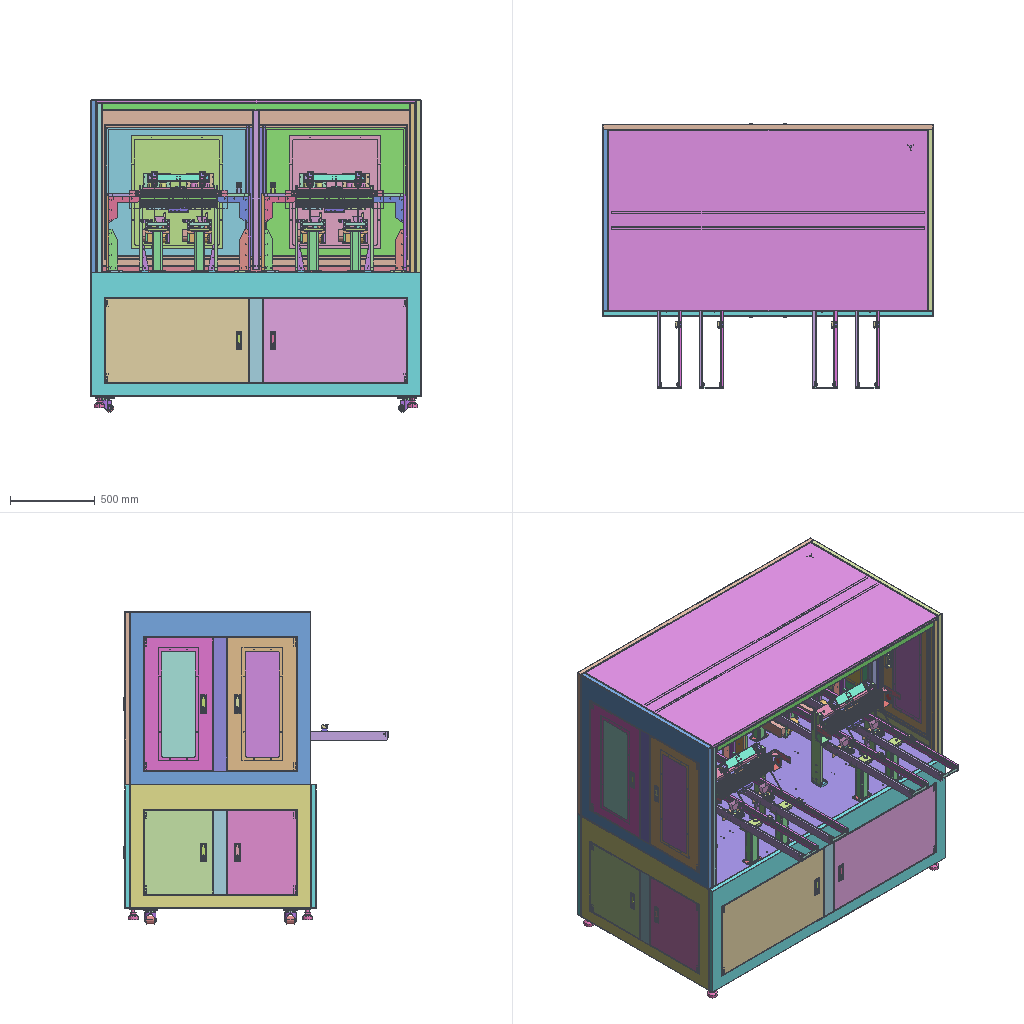Assembly | SolidWorks | 555 different items | 1287 placed | box 1959 x 1559 x 1844 mm
Parts list (item | name | quantity | parent item | size | volume | features), first 326 of 555 items:
1 | 170 Bar Light (subassembly) | x1 | - | - | - | -
2 | (subassembly) | x1 | - | - | - | -
3 | (subassembly) | x1 | - | - | - | -
4 | (subassembly) | x1 | - | - | - | -
5 | (subassembly) | x1 | - | - | - | -
6 | (subassembly) | x1 | - | - | - | -
7 | (subassembly) | x1 | - | - | - | -
8 | (subassembly) | x1 | - | - | - | -
9 | (subassembly) | x1 | - | - | - | -
10 | (subassembly) | x1 | - | - | - | -
11 | (subassembly) | x2 | in 100 | 36 x 22.6 x 446 mm | 126686 mm3 | -
12 | (subassembly) | x1 | - | 36 x 22.6 x 446 mm | 126686 mm3 | -
13 | (subassembly) | x2 | in 102 | 36 x 22.6 x 446 mm | 126686 mm3 | -
14 | (subassembly) | x1 | - | 36 x 22.6 x 446 mm | 126686 mm3 | -
15 | (subassembly) | x2 | in 11 | 36 x 22.6 x 446 mm | 126686 mm3 | -
16 | (subassembly) | x1 | - | 36 x 22.6 x 446 mm | 126686 mm3 | -
17 | (subassembly) | x2 | in 13 | 36 x 22.6 x 446 mm | 126686 mm3 | -
18 | (subassembly) | x1 | - | 36 x 22.6 x 446 mm | 126686 mm3 | -
19 | (subassembly) | x5 | in 41, 42, 106, 107 | 18 x 8 x 56 mm | 2050 mm3 | -
20 | (subassembly) | x5 | in 41, 42, 106, 107 | 18 x 8 x 56 mm | 2050 mm3 | -
21 | (subassembly) | x1 | - | 167.4 x 156.1 x 106 mm | 703605 mm3 | -
22 | (subassembly) | x4 | in 36 | - | 52174 mm3 | -
23 | (subassembly) | x1 | - | - | 52174 mm3 | -
24 | (subassembly) | x1 | - | 54.801 x 54.801 x 36 mm | 20137 mm3 | -
25 | (subassembly) | x1 | - | 26.4 x 61 x 95 mm | 91411 mm3 | -
26 | (subassembly) | x1 | - | 62 x 40 x 105 mm | 103479 mm3 | -
27 | (subassembly) | x4 | in 44 | 110 x 100.5 x 78.14 mm | 89945 mm3 | -
28 | (subassembly) | x4 | in 44 | 40 x 20 x 42 mm | 13632 mm3 | -
29 | (subassembly) | x4 | in 62 | 60 x 143 x 60 mm | 120514 mm3 | -
30 | (subassembly) | x1 | - | 55.81 x 44 x 17.63 mm | 3255 mm3 | -
31 | (subassembly) | x2 | in 34 | - | 422157 mm3 | -
32 | (subassembly) | x4 | in 27 | 29.349 x 29.349 x 44 mm | 30226 mm3 | -
33 | (subassembly) | x4 | in 31 | 39.5 x 98.192 x 39.5 mm | 79084 mm3 | -
34 | (subassembly) | x2 | - | - | 2173391 mm3 | -
35 | (subassembly) | x1 | in 63 | 1886 x 1068 x 18.5 mm | 3707477 mm3 | -
36 | (subassembly) | x4 | in 60 | - | 91199 mm3 | -
37 | (subassembly) | x1 | - | - | 91199 mm3 | -
38 | (subassembly) | x2 | in 58 | 460 x 515 x 80 mm | 1818663 mm3 | -
39 | (subassembly) | x1 | - | 460 x 515 x 80 mm | 1818663 mm3 | features InContextFeatHolder 8
40 | (subassembly) | x2 | in 34 | 380 x 465 x 80 mm | 1262568 mm3 | -
41 | (subassembly) | x1 | in 63 | 851 x 799 x 42.5 mm | 2246546 mm3 | -
42 | (subassembly) | x1 | in 63 | 411 x 799 x 42.5 mm | 1154283 mm3 | -
43 | (subassembly) | x1 | - | 37 x 32 x 81 mm | 32994 mm3 | -
44 | (subassembly) | x4 | - | - | 4376702 mm3 | features Belt 2, AEMSimFeature 1, CompositeCurve 1
45 | (subassembly) | x2 | in 34 | 180 x 151.4 x 77.5 mm | 341470 mm3 | -
46 | (subassembly) | x2 | in 34 | 80 x 78 x 120 mm | 142531 mm3 | -
47 | (subassembly) | x1 | in 62 | 1870 x 1060 x 100 mm | 196301866 mm3 | -
48 | (subassembly) | x20 | in 44 | 26 x 27 x 27 mm | 5259 mm3 | -
49 | (subassembly) | x16 | in 44 | 15 x 27 x 27 mm | 4689 mm3 | -
50 | (subassembly) | x1 | - | 184.199 x 51.718 x 52 mm | 174648 mm3 | features InContextFeatHolder 2
51 | (subassembly) | x2 | in 58 | - | 517771 mm3 | -
52 | (subassembly) | x1 | - | - | 517771 mm3 | -
53 | (subassembly) | x1 | - | - | - | features InContextFeatHolder 9
54 | (subassembly) | x4 | in 62 | 82 x 84 x 107 mm | 193341 mm3 | -
55 | (subassembly) | x1 | - | - | - | features InContextFeatHolder 9
56 | (subassembly) | x1 | - | - | - | features InContextFeatHolder 16
57 | (subassembly) | x1 | - | - | - | features InContextFeatHolder 16
58 | (subassembly) | x2 | - | - | - | features CompositeCurve 1
59 | (subassembly) | x1 | - | - | - | features InContextFeatHolder 4, CompositeCurve 1
60 | (subassembly) | x2 | in 58 | - | 394201 mm3 | features LocalLPattern 1, ReferencePattern 1
61 | (subassembly) | x1 | - | - | 394201 mm3 | features InContextFeatHolder 2, LocalLPattern 1, ReferencePattern 1
62 | (subassembly) | x1 | - | - | 240689348 mm3 | features ReferencePattern 27, LocalLPattern 6, MirrorCompFeat 6
63 | (subassembly) | x1 | in 62 | - | 22995452 mm3 | features ReferencePattern 6, MirrorCompFeat 4
64 | (subassembly) | x2 | in 62 | 1950 x 730 x 42.5 mm | 3302134 mm3 | features MirrorCompFeat 1, ReferencePattern 1
65 | (subassembly) | x1 | - | 195 x 25 x 42 mm | 20018 mm3 | -
66 | (subassembly) | x1 | - | 107.648 x 234.199 x 214.156 mm | 253292 mm3 | features CompositeCurve 1
67 | (subassembly) | x1 | - | 150 x 155 x 181.5 mm | 514877 mm3 | features AEMSimFeature 1
68 | (subassembly) | x2 | in 104 | 306 x 42 x 30 mm | 21853 mm3 | -
69 | (subassembly) | x1 | - | 306 x 42 x 30 mm | 21853 mm3 | -
70 | (subassembly) | x2 | in 100 | 450 x 42 x 35 mm | 35252 mm3 | -
71 | (subassembly) | x1 | - | 450 x 42 x 35 mm | 35252 mm3 | features InContextFeatHolder 2
72 | (subassembly) | x2 | in 97 | 18 x 8 x 56 mm | 2050 mm3 | -
73 | (subassembly) | x1 | in 99 | 18 x 8 x 56 mm | 2050 mm3 | -
74 | (subassembly) | x2 | in 96 | 18 x 8 x 56 mm | 2050 mm3 | -
75 | (subassembly) | x2 | in 92 | 18 x 8 x 56 mm | 2050 mm3 | -
76 | (subassembly) | x2 | in 104 | 36 x 22.6 x 302 mm | 86992 mm3 | -
77 | (subassembly) | x1 | in 91 | 18 x 8 x 56 mm | 2050 mm3 | -
78 | (subassembly) | x1 | in 93 | 18 x 8 x 56 mm | 2050 mm3 | -
79 | (subassembly) | x2 | in 97 | 18 x 8 x 56 mm | 2050 mm3 | -
80 | (subassembly) | x1 | in 99 | 18 x 8 x 56 mm | 2050 mm3 | -
81 | (subassembly) | x2 | in 96 | 18 x 8 x 56 mm | 2050 mm3 | -
82 | (subassembly) | x2 | in 92 | 18 x 8 x 56 mm | 2050 mm3 | -
83 | (subassembly) | x1 | in 91 | 18 x 8 x 56 mm | 2050 mm3 | -
84 | (subassembly) | x1 | in 93 | 18 x 8 x 56 mm | 2050 mm3 | -
85 | (subassembly) | x2 | in 89 | - | 428016 mm3 | -
86 | (subassembly) | x2 | in 85 | 39.5 x 98.192 x 39.5 mm | 82462 mm3 | -
87 | (subassembly) | x1 | - | 36 x 22.6 x 302 mm | 86992 mm3 | -
88 | (subassembly) | x2 | in 85 | 39.5 x 98.192 x 39.5 mm | 82462 mm3 | -
89 | (subassembly) | x2 | - | - | 2167435 mm3 | -
90 | (subassembly) | x2 | in 89 | 380 x 465 x 80 mm | 1262568 mm3 | -
91 | (subassembly) | x1 | in 63 | 851 x 799 x 42.5 mm | 2246546 mm3 | -
92 | (subassembly) | x2 | in 63 | 411 x 799 x 42.5 mm | 1154283 mm3 | -
93 | (subassembly) | x1 | in 63 | 411 x 799 x 42.5 mm | 1154283 mm3 | -
94 | (subassembly) | x2 | in 89 | 180 x 151.4 x 77.5 mm | 341470 mm3 | -
95 | (subassembly) | x2 | in 89 | 80 x 78 x 120 mm | 142531 mm3 | -
96 | (subassembly) | x2 | in 64 | 851 x 509 x 42.5 mm | 870098 mm3 | -
97 | (subassembly) | x2 | in 62 | 411 x 509 x 42.5 mm | 486734 mm3 | -
98 | (subassembly) | x1 | - | 36 x 22.6 x 302 mm | 86992 mm3 | -
99 | (subassembly) | x1 | in 62 | 411 x 509 x 42.5 mm | 486734 mm3 | -
100 | (subassembly) | x2 | in 51 | - | 230759 mm3 | -
101 | (subassembly) | x1 | - | - | 230759 mm3 | -
102 | (subassembly) | x2 | in 51 | - | 224548 mm3 | -
103 | (subassembly) | x1 | - | - | 224548 mm3 | -
104 | (subassembly) | x2 | in 51 | 306 x 50.679 x 130.275 mm | 162971 mm3 | -
105 | (subassembly) | x1 | - | 306 x 50.679 x 130.275 mm | 162971 mm3 | -
106 | (subassembly) | x2 | in 64 | 851 x 509 x 42.5 mm | 870098 mm3 | -
107 | (subassembly) | x1 | in 62 | 411 x 509 x 42.5 mm | 486734 mm3 | -
108 | - | x1 | - | 1386 x 30 x 15 mm | 332572 mm3 | features HoleWzd 2, 3DProfileFeature 1, ICE 1, WeldMemberFeat 1, WeldmentFeature 1
109 | - | x4 | in 28 | 12 x 11 x 15 mm | 1507 mm3 | features ICE 5, Chamfer 2, Extrusion 1
110 | - | x4 | in 28 | 40 x 20 x 16 mm | 7506 mm3 | features HoleWzd 2, Chamfer 1, Extrusion 1, ICE 1
111 | - | x1 | - | 1087 x 374 x 123 mm | 809461 mm3 | features ICE 4, Fillet 2, EdgeFlange 1, FlatPattern 1, SMBaseFlange 1, SheetMetal 1
112 | - | x1 | - | 1087 x 374 x 1.5 mm | 609421 mm3 | features Fillet 1, FlatPattern 1, ICE 1, SMBaseFlange 1, SheetMetal 1
113 | - | x1 | - | 1280 x 374 x 1.5 mm | 717635 mm3 | features Fillet 1, FlatPattern 1, HoleWzd 1, SMBaseFlange 1, SheetMetal 1
114 | - | x1 | - | 10 x 145 x 145 mm | 203124 mm3 | features HoleWzd 2, ICE 2, Chamfer 1, Extrusion 1
115 | - | x1 | - | 100 x 301.5 x 60 mm | 406752 mm3 | features Chamfer 4, ICE 4, HoleWzd 2, 3DProfileFeature 1, WeldMemberFeat 1, WeldmentFeature 1
116 | - | x1 | - | 20 x 410 x 40 mm | 242107 mm3 | features ICE 3, Chamfer 1, Extrusion 1, HoleWzd 1
117 | - | x1 | - | 317 x 30 x 11 mm | 98288 mm3 | features Chamfer 2, HoleWzd 2, Extrusion 1, ICE 1
118 | - | x1 | - | 317 x 15 x 170 mm | 619521 mm3 | features ICE 5, HoleWzd 4, Chamfer 2, Extrusion 1, Fillet 1
119 | - | x1 | - | 805 x 30 x 15 mm | 189619 mm3 | features 3DProfileFeature 1, HoleWzd 1, ICE 1, WeldMemberFeat 1, WeldmentFeature 1
120 | - | x1 | - | 317 x 8 x 29 mm | 69848 mm3 | features HoleWzd 2, ICE 2, Chamfer 1, Extrusion 1
121 | - | x1 | - | 297 x 3 x 90 mm | 79946 mm3 | features Chamfer 3, Extrusion 1, HoleWzd 1
122 | - | x1 | - | 30 x 30 x 10 mm | 7510 mm3 | features Chamfer 2, Extrusion 1, HoleWzd 1, ICE 1
123 | - | x1 | - | 18 x 14 x 15 mm | 1893 mm3 | features ICE 2, Chamfer 1, Extrusion 1, HoleWzd 1
124 | - | x1 | - | 62 x 8 x 20 mm | 9069 mm3 | features Chamfer 1, Extrusion 1, HoleWzd 1
125 | - | x1 | - | 20 x 20 x 415 mm | 128650 mm3 | features HoleWzd 2, Chamfer 1, Extrusion 1
126 | - | x1 | - | 210 x 12 x 280 mm | 525634 mm3 | features ICE 4, Chamfer 3, Extrusion 1, Fillet 1
127 | - | x1 | - | 35 x 15 x 40 mm | 12452 mm3 | features Chamfer 1, Extrusion 1, HoleWzd 1, ICE 1
128 | - | x1 | - | 48 x 133 x 30 mm | 14568 mm3 | features CornerTrim 2, ICE 2, FlatPattern 1, HoleWzd 1, SMBaseFlange 1, SheetMetal 1
129 | - | x1 | - | 50 x 30 x 15 mm | 18955 mm3 | features Chamfer 2, Extrusion 1, HoleWzd 1
130 | - | x1 | - | 1386 x 30 x 15 mm | 334202 mm3 | features 3DProfileFeature 1, HoleWzd 1, ICE 1, WeldMemberFeat 1, WeldmentFeature 1
131 | - | x1 | - | 50 x 30 x 15 mm | 18955 mm3 | features Chamfer 2, Extrusion 1, HoleWzd 1
132 | - | x1 | - | 40 x 30 x 15 mm | 15105 mm3 | features Chamfer 1, Extrusion 1, HoleWzd 1
133 | - | x1 | - | 20 x 16 x 20 mm | 4067 mm3 | features HoleWzd 2, Chamfer 1, Extrusion 1, ICE 1
134 | - | x1 | - | 20 x 16 x 20 mm | 4064 mm3 | features HoleWzd 2, Chamfer 1, Extrusion 1, ICE 1
135 | - | x1 | - | 28 x 12 x 18 mm | 4573 mm3 | features Chamfer 1, Extrusion 1, HoleWzd 1
136 | - | x1 | - | 330 x 10 x 30 mm | 97693 mm3 | features Chamfer 1, Extrusion 1, HoleWzd 1
137 | - | x1 | - | 30 x 40 x 40 mm | 21456 mm3 | features Chamfer 3, ICE 2, Extrusion 1, HoleWzd 1
138 | - | x1 | - | 40 x 320 x 40 mm | 193550 mm3 | features WeldMemberFeat 1, WeldmentFeature 1
139 | - | x1 | - | 39 x 35 x 33 mm | 21329 mm3 | features HoleWzd 2, Chamfer 1, Extrusion 1, ICE 1
140 | - | x1 | - | 16.5 x 26.5 x 35 mm | 1824 mm3 | features ICE 2, Chamfer 1, FlatPattern 1, SMBaseFlange 1, SheetMetal 1
141 | - | x1 | - | 805 x 30 x 15 mm | 190827 mm3 | features 3DProfileFeature 1, HoleWzd 1, ICE 1, WeldMemberFeat 1, WeldmentFeature 1
142 | - | x1 | - | 50 x 5 x 30 mm | 6223 mm3 | features ICE 3, Chamfer 2, HoleWzd 2, CornerTrim 1, FlatPattern 1, SMBaseFlange 1, SheetMetal 1
143 | - | x1 | - | 1283 x 1093 x 1.5 mm | 2101440 mm3 | features HoleWzd 2, Cut 1, Extrusion 1, Fillet 1
144 | - | x1 | - | 30 x 40 x 200 mm | 67180 mm3 | features Chamfer 2, HoleWzd 2, Extrusion 1, ICE 1
145 | - | x1 | - | 140 x 539 x 60 mm | 688528 mm3 | features Chamfer 3, ICE 3, HoleWzd 2, 3DProfileFeature 1, WeldMemberFeat 1, WeldmentFeature 1
146 | - | x1 | - | 1000 x 60 x 20 mm | 1185060 mm3 | features Chamfer 2, HoleWzd 2, Extrusion 1, LPattern 1
147 | - | x1 | - | 80 x 379 x 120 mm | 535710 mm3 | features HoleWzd 4, Chamfer 2, ICE 2, WeldMemberFeat 1, WeldmentFeature 1
148 | - | x1 | - | 633 x 12 x 86.5 mm | 646529 mm3 | features HoleWzd 6, Cut 5, ICE 3, Chamfer 2, LPattern 2, Extrusion 1
149 | - | x1 | - | 680 x 45 x 10 mm | 288393 mm3 | features HoleWzd 10, Chamfer 2, Cut 1, Extrusion 1, LPattern 1
150 | - | x1 | - | 64 x 102 x 19 mm | 119355 mm3 | features HoleWzd 4, Chamfer 2, Cut 1, Extrusion 1, ICE 1
151 | - | x1 | - | 130 x 84 x 12 mm | 83062 mm3 | features ICE 8, Chamfer 3, HoleWzd 3, Cut 2, Extrusion 1
152 | - | x1 | - | 10 x 14 x 10 mm | 408.891 mm3 | features Chamfer 3, ICE 3, Extrusion 1
153 | - | x1 | - | 72 x 98 x 40 mm | 71413 mm3 | features HoleWzd 3, Chamfer 2, Cut 1, Extrusion 1, Fillet 1
154 | - | x1 | - | 50 x 30 x 10 mm | 12561 mm3 | features HoleWzd 2, Chamfer 1, Extrusion 1
155 | - | x1 | - | 42 x 59 x 21 mm | 26880 mm3 | features ICE 4, Chamfer 2, HoleWzd 2, Extrusion 1
156 | - | x1 | - | 20 x 19.9 x 54 mm | 6398 mm3 | features ICE 8, HoleWzd 3, Extrusion 1
157 | - | x1 | - | 30 x 24.5 x 29.5 mm | 1040 mm3 | features Fillet 3, ICE 3, EdgeFlange 2, Cut 1, FlatPattern 1, SMBaseFlange 1, SheetMetal 1
158 | - | x1 | - | 110 x 85 x 4 mm | 36598 mm3 | features HoleWzd 2, Chamfer 1, Extrusion 1
159 | - | x1 | - | 110 x 85 x 2 mm | 15306 mm3 | features ICE 15, HoleWzd 5, MoveFace 2, Chamfer 1, Cut 1, Extrusion 1, Fillet 1, MirrorPattern 1
160 | - | x1 | - | 30 x 85 x 29 mm | 7084 mm3 | features EdgeFlange 3, HoleWzd 2, FlatPattern 1, SMBaseFlange 1, SheetMetal 1
161 | - | x1 | - | 77 x 33 x 22 mm | 5955 mm3 | features EdgeFlange 2, HoleWzd 2, Chamfer 1, FlatPattern 1, ICE 1, SMBaseFlange 1, SheetMetal 1
162 | - | x1 | - | 64 x 14 x 87 mm | 75198 mm3 | features HoleWzd 2, Chamfer 1, Extrusion 1
163 | - | x2 | in 104 | 120 x 128.5 x 45 mm | 54126 mm3 | features HoleWzd 3, EdgeFlange 2, Fillet 1, FlatPattern 1, ICE 1, SMBaseFlange 1, SheetMetal 1
164 | - | x1 | - | 8 x 70 x 8 mm | 3389 mm3 | features Chamfer 1, Extrusion 1, HoleWzd 1
165 | - | x1 | - | 10 x 90 x 58 mm | 50238 mm3 | features HoleWzd 2, Chamfer 1, Extrusion 1
166 | - | x1 | - | 110 x 85 x 4 mm | 36664 mm3 | features HoleWzd 2, Chamfer 1, Extrusion 1
167 | - | x1 | - | 24 x 8 x 170 mm | 30923 mm3 | features Chamfer 2, HoleWzd 2, Extrusion 1
168 | - | x1 | - | 110 x 85 x 6 mm | 53736 mm3 | features HoleWzd 2, Chamfer 1, Extrusion 1
169 | - | x1 | - | 64 x 130 x 10 mm | 78799 mm3 | features HoleWzd 2, Chamfer 1, Extrusion 1
170 | - | x1 | - | 74 x 216 x 12 mm | 104830 mm3 | features Chamfer 2, HoleWzd 2, Cut 1, Extrusion 1
171 | - | x1 | - | 12 x 68 x 33 mm | 24708 mm3 | features HoleWzd 3, Chamfer 1, Extrusion 1
172 | - | x1 | - | 25 x 36 x 10 mm | 6742 mm3 | features HoleWzd 2, Chamfer 1, Extrusion 1
173 | - | x1 | - | 60 x 72 x 12 mm | 45188 mm3 | features HoleWzd 2, Chamfer 1, Extrusion 1
174 | - | x1 | - | 120 x 128.5 x 45 mm | 54126 mm3 | features HoleWzd 3, EdgeFlange 2, Fillet 1, FlatPattern 1, ICE 1, SMBaseFlange 1, SheetMetal 1
175 | - | x1 | - | 870 x 90 x 10 mm | 777394 mm3 | features HoleWzd 4, Chamfer 1, Extrusion 1, ICE 1, LPattern 1
176 | - | x1 | - | 20 x 20 x 4 mm | 1002 mm3 | features Extrusion 1
177 | - | x1 | - | 12 x 28 x 68 mm | 21134 mm3 | features Chamfer 2, HoleWzd 2, Extrusion 1
178 | - | x1 | - | 110 x 85 x 2 mm | 15729 mm3 | features Cut 2, Extrusion 1
179 | - | x4 | in 44 | 20 x 50 x 1500 mm | 1167448 mm3 | features HoleWzd 7, Cut 3, Chamfer 2, ICE 2, Extrusion 1, Fillet 1
180 | - | x8 | in 44 | 100 x 250.5 x 60 mm | 355325 mm3 | features Chamfer 2, HoleWzd 2, ICE 2, 3DProfileFeature 1, WeldMemberFeat 1, WeldmentFeature 1
181 | - | x8 | in 44 | 60 x 13 x 144 mm | 107062 mm3 | features HoleWzd 2, Chamfer 1, Extrusion 1
182 | - | x4 | in 44 | 20 x 50 x 1500 mm | 1170334 mm3 | features HoleWzd 7, ICE 4, Chamfer 2, Extrusion 1, Fillet 1
183 | - | x4 | in 44 | 144 x 35 x 5 mm | 17146 mm3 | features Chamfer 1, Extrusion 1, Fillet 1, HoleWzd 1, ICE 1
184 | - | x4 | in 44 | 30 x 33 x 144 mm | 12527 mm3 | features Fillet 3, ICE 2, Cut 1, Extrusion 1, Shell 1
185 | - | x5 | in 41, 42, 106, 107 | 35 x 42.5 x 110 mm | 68844 mm3 | features BaseBody 1
186 | - | x2 | in 15 | 36 x 15 x 6 mm | 2540 mm3 | features BaseBody 1
187 | - | x1 | - | 36 x 15 x 6 mm | 2540 mm3 | features BaseBody 1
188 | - | x2 | in 17 | 36 x 15 x 6 mm | 2540 mm3 | features BaseBody 1
189 | - | x1 | - | 36 x 15 x 6 mm | 2540 mm3 | features BaseBody 1
190 | - | x2 | in 76 | 36 x 15 x 6 mm | 2540 mm3 | features BaseBody 1
191 | - | x1 | - | 36 x 15 x 6 mm | 2540 mm3 | features BaseBody 1
192 | - | x1 | - | 36 x 15 x 6 mm | 2540 mm3 | features BaseBody 1
193 | - | x2 | in 15 | 36 x 15 x 6 mm | 2606 mm3 | features BaseBody 1
194 | - | x1 | - | 36 x 15 x 6 mm | 2606 mm3 | features BaseBody 1
195 | - | x2 | in 17 | 36 x 15 x 6 mm | 2606 mm3 | features BaseBody 1
196 | - | x1 | - | 40 x 40 x 35 mm | 11668 mm3 | features ICE 3, Extrusion 1
197 | - | x1 | - | 36 x 15 x 6 mm | 2606 mm3 | features BaseBody 1
198 | - | x2 | in 76 | 36 x 15 x 6 mm | 2606 mm3 | features BaseBody 1
199 | - | x1 | - | 36 x 15 x 6 mm | 2606 mm3 | features BaseBody 1
200 | - | x1 | - | 36 x 15 x 6 mm | 2606 mm3 | features BaseBody 1
201 | - | x2 | in 45 | 174 x 1 x 62.5 mm | 10875 mm3 | features BaseBody 1
202 | - | x2 | in 45 | 5 x 105.4 x 62 mm | 29217 mm3 | features BaseBody 1
203 | - | x2 | in 45 | 177 x 36.8 x 1 mm | 6475 mm3 | features BaseBody 1
204 | - | x2 | in 45 | 5 x 105.4 x 62 mm | 29184 mm3 | features BaseBody 1
205 | - | x2 | in 45 | 174 x 6 x 62 mm | 63958 mm3 | features BaseBody 1
206 | - | x2 | in 45 | 174 x 6 x 62 mm | 62898 mm3 | features BaseBody 1
207 | - | x4 | in 100 | 260 x 40 x 130 mm | 34410 mm3 | features HoleWzd 3, EdgeFlange 1, Fillet 1, FlatPattern 1, ICE 1, SMBaseFlange 1, SheetMetal 1
208 | - | x2 | in 45 | 180 x 105.4 x 6 mm | 51969 mm3 | features BaseBody 1
209 | - | x2 | in 45 | 174 x 3 x 62.5 mm | 32625 mm3 | features BaseBody 1
210 | - | x2 | in 45 | 172 x 61 x 61 mm | 14666 mm3 | features BaseBody 1
211 | - | x1 | - | 42 x 17 x 17 mm | 8111 mm3 | features BaseBody 1
212 | - | x4 | in 44 | 16 x 32.358 x 32.358 mm | 6392 mm3 | features ICE 1, Revolution 1
213 | - | x4 | in 44 | 16 x 32.358 x 32.358 mm | 5839 mm3 | features ICE 1, Revolution 1
214 | - | x1 | - | 114 x 47 x 26 mm | 54432 mm3 | features BaseBody 1
215 | - | x1 | - | 158 x 46 x 18 mm | 18569 mm3 | features BaseBody 5
216 | - | x4 | in 33 | 52.8 x 39.5 x 39.5 mm | 57776 mm3 | features Extrusion 1, ICE 1
217 | - | x4 | in 29 | 60 x 143 x 60 mm | 112312 mm3 | features BaseBody 1
218 | - | x1 | - | 39 x 29.5 x 121 mm | 53131 mm3 | features RefAxis 15, HoleWzd 11, ICE 9, 3DProfileFeature 5, LPattern 4, Revolution 3, RevCut 2, Extrusion 1
219 | - | x1 | - | 260 x 40 x 130 mm | 34410 mm3 | features HoleWzd 3, EdgeFlange 1, Fillet 1, FlatPattern 1, ICE 1, SMBaseFlange 1, SheetMetal 1
220 | - | x4 | in 29 | 30 x 16 x 34.641 mm | 8202 mm3 | features BaseBody 1
221 | - | x1 | - | 16.782 x 16 x 17.8 mm | 1225 mm3 | features ICE 4, RefAxis 3, 3DProfileFeature 1, Extrusion 1, Revolution 1
222 | - | x1 | - | 19 x 82 x 28.4 mm | 14487 mm3 | features ICE 12, RefAxis 3, 3DProfileFeature 1, Extrusion 1, Revolution 1
223 | - | x1 | - | 7.2 x 34.2 x 43.1 mm | 5332 mm3 | features RefAxis 9, 3DProfileFeature 3, ICE 2, Extrusion 1
224 | - | x1 | - | 9 x 12 x 9 mm | 395.605 mm3 | features RefAxis 6, 3DProfileFeature 2, Revolution 1
225 | - | x1 | - | 9.996 x 20 x 10 mm | 691.38 mm3 | features BaseBody 1
226 | - | x1 | - | 8 x 32 x 8 mm | 1009 mm3 | features RefAxis 12, 3DProfileFeature 4, Revolution 2, ICE 1, RevCut 1
227 | - | x1 | - | 13.856 x 3 x 12 mm | 252.9 mm3 | features RefAxis 3, 3DProfileFeature 1, ICE 1, Revolution 1
228 | - | x1 | - | 55 x 2 x 14 mm | 1344 mm3 | features RefAxis 3, 3DProfileFeature 1, Extrusion 1
229 | - | x2 | in 76 | 36 x 22.6 x 302 mm | 68970 mm3 | features BaseBody 1
230 | - | x1 | - | 97 x 56.4 x 56.4 mm | 215664 mm3 | features ICE 4, Fillet 2, CirPattern 1, Extrusion 1
231 | - | x1 | - | 36 x 22.6 x 302 mm | 68970 mm3 | features BaseBody 1
232 | - | x1 | - | 36 x 22.6 x 302 mm | 68970 mm3 | features BaseBody 1
233 | - | x2 | in 76 | 31.173 x 7.2 x 23.95 mm | 1073 mm3 | features BaseBody 1
234 | - | x1 | - | 31.173 x 7.2 x 23.95 mm | 1073 mm3 | features BaseBody 1
235 | - | x1 | - | 31.173 x 7.2 x 23.95 mm | 1073 mm3 | features BaseBody 1
236 | - | x2 | in 76 | 31.173 x 7.2 x 23.95 mm | 1073 mm3 | features BaseBody 1
237 | - | x1 | - | 31.173 x 7.2 x 23.95 mm | 1073 mm3 | features BaseBody 1
238 | - | x1 | - | 31.173 x 7.2 x 23.95 mm | 1073 mm3 | features BaseBody 1
239 | - | x2 | in 76 | 31.173 x 7.2 x 23.95 mm | 1073 mm3 | features BaseBody 1
240 | - | x1 | - | 31.173 x 7.2 x 23.95 mm | 1073 mm3 | features BaseBody 1
241 | - | x1 | - | 53 x 45.8 x 53.4 mm | 95835 mm3 | features ICE 7, RefAxis 6, HoleWzd 3, 3DProfileFeature 2, Extrusion 1, LPattern 1, Revolution 1
242 | - | x1 | - | 31.173 x 7.2 x 23.95 mm | 1073 mm3 | features BaseBody 1
243 | - | x2 | in 76 | 31.173 x 7.2 x 23.95 mm | 1073 mm3 | features BaseBody 1
244 | - | x1 | - | 31.173 x 7.2 x 23.95 mm | 1073 mm3 | features BaseBody 1
245 | - | x1 | - | 31.173 x 7.2 x 23.95 mm | 1073 mm3 | features BaseBody 1
246 | - | x2 | in 76 | 31.173 x 7.2 x 23.95 mm | 1073 mm3 | features BaseBody 1
247 | - | x1 | - | 31.173 x 7.2 x 23.95 mm | 1073 mm3 | features BaseBody 1
248 | - | x1 | - | 31.173 x 7.2 x 23.95 mm | 1073 mm3 | features BaseBody 1
249 | - | x2 | in 76 | 31.173 x 7.2 x 23.95 mm | 1073 mm3 | features BaseBody 1
250 | - | x1 | - | 31.173 x 7.2 x 23.95 mm | 1073 mm3 | features BaseBody 1
251 | - | x1 | - | 31.173 x 7.2 x 23.95 mm | 1073 mm3 | features BaseBody 1
252 | - | x1 | - | 19.5 x 11 x 8 mm | 1100 mm3 | features RefAxis 3, Revolution 2, 3DProfileFeature 1, Extrusion 1, HoleWzd 1
253 | - | x2 | in 76 | 31.173 x 7.2 x 23.95 mm | 1073 mm3 | features BaseBody 1
254 | - | x1 | - | 31.173 x 7.2 x 23.95 mm | 1073 mm3 | features BaseBody 1
255 | - | x1 | - | 31.173 x 7.2 x 23.95 mm | 1073 mm3 | features BaseBody 1
256 | - | x2 | in 76 | 31.173 x 7.2 x 23.95 mm | 1073 mm3 | features BaseBody 1
257 | - | x1 | - | 31.173 x 7.2 x 23.95 mm | 1073 mm3 | features BaseBody 1
258 | - | x1 | - | 31.173 x 7.2 x 23.95 mm | 1073 mm3 | features BaseBody 1
259 | - | x2 | in 76 | 31.173 x 7.2 x 23.95 mm | 1073 mm3 | features BaseBody 1
260 | - | x1 | - | 31.173 x 7.2 x 23.95 mm | 1073 mm3 | features BaseBody 1
261 | - | x1 | - | 31.173 x 7.2 x 23.95 mm | 1073 mm3 | features BaseBody 1
262 | - | x2 | in 76 | 31.173 x 7.2 x 23.95 mm | 1073 mm3 | features BaseBody 1
263 | - | x1 | - | 46 x 74.3 x 53 mm | 114802 mm3 | features RefAxis 6, ICE 4, 3DProfileFeature 2, Revolution 1
264 | - | x1 | - | 31.173 x 7.2 x 23.95 mm | 1073 mm3 | features BaseBody 1
265 | - | x1 | - | 31.173 x 7.2 x 23.95 mm | 1073 mm3 | features BaseBody 1
266 | - | x2 | in 76 | 31.173 x 7.2 x 23.95 mm | 1073 mm3 | features BaseBody 1
267 | - | x1 | - | 31.173 x 7.2 x 23.95 mm | 1073 mm3 | features BaseBody 1
268 | - | x1 | - | 31.173 x 7.2 x 23.95 mm | 1073 mm3 | features BaseBody 1
269 | - | x2 | in 76 | 31.173 x 7.2 x 23.95 mm | 1073 mm3 | features BaseBody 1
270 | - | x1 | - | 31.173 x 7.2 x 23.95 mm | 1073 mm3 | features BaseBody 1
271 | - | x1 | - | 31.173 x 7.2 x 23.95 mm | 1073 mm3 | features BaseBody 1
272 | - | x1 | - | 120 x 120 x 38.5 mm | 90385 mm3 | features ICE 3, CirPattern 1, Extrusion 1, Fillet 1, HoleWzd 1, MirrorPattern 1
273 | - | x4 | in 32 | 29.349 x 29.349 x 40.5 mm | 29191 mm3 | features RevCut 4, Extrusion 1, ICE 1
274 | - | x1 | - | 53 x 69.9 x 53.4 mm | 106071 mm3 | features ICE 11, RefAxis 6, HoleWzd 3, 3DProfileFeature 2, Revolution 2, Extrusion 1, LPattern 1
275 | - | x4 | in 36 | 36.008 x 31 x 53.1 mm | 39029 mm3 | features MBimport 1
276 | - | x1 | - | 36.008 x 31 x 53.1 mm | 39029 mm3 | features MBimport 1
277 | - | x4 | in 33 | - | - | features BaseBody 9, RefSurface 2
278 | - | x4 | in 32 | 8 x 8 x 22.5 mm | 1035 mm3 | features ICE 1, RevCut 1, Revolution 1
279 | - | x1 | in 63 | 1950 x 1020 x 48.5 mm | 1634883 mm3 | features EdgeFlange 5, FlatPattern 1, HoleWzd 1, ICE 1, SMBaseFlange 1, SheetMetal 1
280 | - | x1 | in 35 | 1886 x 1068 x 18.5 mm | 3323198 mm3 | features EdgeFlange 2, HoleWzd 2, CirPattern 1, FlatPattern 1, SMBaseFlange 1, SheetMetal 1
281 | - | x1 | in 35 | 110 x 17 x 1845 mm | 384278 mm3 | features FlatPattern 1, SMBaseFlange 1, SheetMetal 1
282 | - | x2 | in 38 | 430 x 80 x 15 mm | 509108 mm3 | features HoleWzd 5, Extrusion 1, MirrorPattern 1
283 | - | x1 | - | 430 x 80 x 15 mm | 509108 mm3 | features HoleWzd 5, Extrusion 1, MirrorPattern 1
284 | - | x4 | in 38 | 80 x 500 x 15 mm | 549882 mm3 | features HoleWzd 4, Extrusion 1, Fillet 1, MirrorPattern 1
285 | - | x1 | - | 46 x 74.3 x 53 mm | 114802 mm3 | features ICE 4, RefAxis 3, 3DProfileFeature 1, Revolution 1
286 | - | x1 | - | 80 x 500 x 15 mm | 549882 mm3 | features HoleWzd 4, Extrusion 1, Fillet 1, MirrorPattern 1
287 | - | x2 | in 40 | 80 x 450 x 15 mm | 533651 mm3 | features HoleWzd 4, Extrusion 1
288 | - | x2 | in 40 | 365 x 80 x 15 mm | 415130 mm3 | features HoleWzd 6, Extrusion 1
289 | - | x1 | - | 238.5 x 96 x 130.5 mm | 1680517 mm3 | features ICE 5, Extrusion 1, Fillet 1
290 | - | x1 | - | 25 x 440 x 25 mm | 214356 mm3 | features Chamfer 1, Extrusion 1, HoleWzd 1
291 | - | x2 | in 15 | 36 x 22.6 x 446 mm | 102225 mm3 | features BaseBody 1
292 | - | x1 | - | 36 x 22.6 x 446 mm | 102225 mm3 | features BaseBody 1
293 | - | x2 | in 17 | 36 x 22.6 x 446 mm | 102225 mm3 | features BaseBody 1
294 | - | x1 | - | 36 x 22.6 x 446 mm | 102225 mm3 | features BaseBody 1
295 | - | x1 | in 62 | 1070 x 730 x 30 mm | 905404 mm3 | features EdgeFlange 4, FlatPattern 1, HoleWzd 1, ICE 1, SMBaseFlange 1, SheetMetal 1
296 | - | x1 | - | 53 x 48.5 x 57 mm | 88299 mm3 | features ICE 8, RefAxis 6, HoleWzd 3, 3DProfileFeature 2, Extrusion 1, RevCut 1, Revolution 1
297 | - | x1 | in 63 | 1070 x 1020 x 48.5 mm | 1078277 mm3 | features EdgeFlange 5, FlatPattern 1, HoleWzd 1, ICE 1, SMBaseFlange 1, SheetMetal 1
298 | - | x4 | in 22 | 4 x 180 x 4 mm | 2262 mm3 | features Extrusion 1
299 | - | x1 | - | 4 x 180 x 4 mm | 2262 mm3 | features Extrusion 1
300 | - | x4 | in 60 | 4 x 300 x 4 mm | 3770 mm3 | features Extrusion 1
301 | - | x1 | - | 4 x 300 x 4 mm | 3770 mm3 | features Extrusion 1
302 | - | x1 | in 41 | 851 x 786 x 26.5 mm | 735444 mm3 | features ICE 4, EdgeFlange 2, MirrorPattern 2, Fillet 1, FlatPattern 1, HoleWzd 1, SMBaseFlange 1, SheetMetal 1
303 | - | x1 | in 42 | 411 x 786 x 26.5 mm | 442380 mm3 | features ICE 4, EdgeFlange 2, MirrorPattern 2, Fillet 1, FlatPattern 1, HoleWzd 1, SMBaseFlange 1, SheetMetal 1
304 | - | x4 | in 44 | 70 x 70 x 144 mm | 464406 mm3 | features ICE 3, Fillet 2, Extrusion 1, HoleWzd 1
305 | - | x1 | - | 19 x 50 x 62 mm | 31201 mm3 | features Extrusion 1, Fillet 1, HoleWzd 1
306 | - | x1 | - | 19 x 50 x 62 mm | 31201 mm3 | features Extrusion 1, Fillet 1, HoleWzd 1
307 | - | x1 | - | 53 x 64.2 x 57 mm | 112882 mm3 | features RefAxis 6, ICE 3, 3DProfileFeature 2, Revolution 2, Extrusion 1, LPattern 1
308 | - | x1 | - | 19 x 50 x 62 mm | 31201 mm3 | features Extrusion 1, Fillet 1, HoleWzd 1
309 | - | x2 | in 46 | 8 x 70 x 120 mm | 59993 mm3 | features HoleWzd 3, Chamfer 2, Extrusion 1, ICE 1
310 | - | x2 | in 46 | 8 x 80 x 120 mm | 61128 mm3 | features HoleWzd 3, Extrusion 1, Fillet 1, MirrorPattern 1
311 | - | x2 | in 60 | 8 x 50 x 320 mm | 127555 mm3 | features Extrusion 1, Fillet 1, HoleWzd 1
312 | - | x1 | - | 8 x 50 x 320 mm | 127555 mm3 | features Extrusion 1, Fillet 1, HoleWzd 1
313 | - | x2 | in 31 | 28 x 120 x 160 mm | 167009 mm3 | features HoleWzd 4, ICE 3, Extrusion 1
314 | - | x1 | - | 40 x 1203 x 40 mm | 719325 mm3 | features ICE 1, WeldMemberFeat 1, WeldmentFeature 1
315 | - | x1 | - | 40 x 1467 x 40 mm | 887305 mm3 | features WeldMemberFeat 1, WeldmentFeature 1
316 | - | x1 | - | 40 x 140 x 40 mm | 83784 mm3 | features HoleWzd 1, WeldMemberFeat 1, WeldmentFeature 1
317 | - | x1 | - | 40 x 340 x 40 mm | 205625 mm3 | features HoleWzd 1, WeldMemberFeat 1, WeldmentFeature 1
318 | - | x1 | - | 37.5 x 37.5 x 40.5 mm | 27726 mm3 | features RefAxis 3, Revolution 2, 3DProfileFeature 1, ICE 1
319 | - | x1 | - | 40 x 413 x 40 mm | 248012 mm3 | features HoleWzd 1, WeldMemberFeat 1, WeldmentFeature 1
320 | - | x1 | - | 40 x 540 x 40 mm | 323932 mm3 | features HoleWzd 1, WeldMemberFeat 1, WeldmentFeature 1
321 | - | x1 | - | 40 x 1013 x 40 mm | 612706 mm3 | features WeldMemberFeat 1, WeldmentFeature 1
322 | - | x1 | - | 40 x 580 x 40 mm | 350809 mm3 | features WeldMemberFeat 1, WeldmentFeature 1
323 | - | x4 | in 62 | 40 x 40 x 10 mm | 15637 mm3 | features Extrusion 1, HoleWzd 1
324 | - | x1 | in 62 | 107 x 162 x 10 mm | 168631 mm3 | features HoleWzd 2, Extrusion 1, Fillet 1, LPattern 1
325 | - | x2 | in 62 | 40 x 40 x 10 mm | 15637 mm3 | features Extrusion 1, HoleWzd 1
326 | - | x2 | in 62 | 40 x 40 x 10 mm | 15637 mm3 | features Extrusion 1, HoleWzd 1
Mates (type | each side: item.copy, entity, surface, feature), first 317 of 520 lines:
In the top assembly
Coincident | 334.1 face plane Boss-Extrude 1 | 180.1 face plane Boss-Extrude 2
DistanceDim | 179.1 face plane Boss-Extrude 1 | 295.1 face plane Base-Flange 1
DistanceDim | 182.1 face plane Boss-Extrude 4 | 279.1 face plane Base-Flange 1
Coincident | 334.1 face plane Boss-Extrude 1 | 368.1 face plane Boss-Extrude 1
DistanceDim | 287.1 face plane Boss-Extrude 1 | 179.1 face plane Boss-Extrude 1
DistanceDim | 368.1 face plane Boss-Extrude 1 | 360.1 face plane Base-Flange 1
Coincident | 334.1 face plane Boss-Extrude 1 | 366.1 face plane Boss-Extrude 1
Width | 284.1 face plane Boss-Extrude 1 | 284.2 face plane Boss-Extrude 1 | 179.1 face plane Boss-Extrude 1 | 182.2 face plane Boss-Extrude 1
DistanceDim | 284.2 face plane Boss-Extrude 1 | 360.1 face plane Base-Flange 1
In subassembly 34
DistanceDim | 208.1 face plane Import 1 | 309.1 face plane Boss-Extrude 1
Coincident | 288.1 face plane Boss-Extrude 1 | 313.1 face plane Boss-Extrude 1 | 3 times
Coincident | 288.1 face plane Boss-Extrude 1 | 309.1 face plane Boss-Extrude 1
DistanceDim | 310.1 face plane Boss-Extrude 1 | 288.1 face plane Boss-Extrude 1
Coincident | 288.1 face plane Boss-Extrude 1 | 34.1 face
DistanceDim | 34.1 face | 288.1 face plane Boss-Extrude 1
DistanceDim | 313.1 face plane Boss-Extrude 1 | 34.1 face
Width | 310.1 face plane Boss-Extrude 1 | 310.1 face plane Boss-Extrude 1 | 313.1 face plane Boss-Extrude 1 | 313.1 face plane Boss-Extrude 1
Coincident | 205.1 face plane Import 1 | 310.1 face plane Boss-Extrude 1
Width | 208.1 face plane Import 1 | 208.1 face plane Import 1 | 310.1 face plane Boss-Extrude 1 | 310.1 face plane Boss-Extrude 1
In subassembly 46
DistanceDim | 309.2 face plane Boss-Extrude 1 | 310.2 face plane Boss-Extrude 1
Concentric | 309.2 face cylinder M4 Tapped Hole 1 | 310.2 face cylinder M4 Socket Head Cap Screw Counterbore Hole 4 | 2 times
Width | 365.1 face plane Boss-Extrude 1 | 365.1 face plane Boss-Extrude 1 | 310.2 face plane M4 Socket Head Cap Screw Counterbore Hole 11 | 310.2 face plane M4 Socket Head Cap Screw Counterbore Hole 11
Coincident | 309.2 face plane Boss-Extrude 1 | 365.1 face plane Boss-Extrude 1
Coincident | 310.2 face plane Boss-Extrude 1 | 365.1 face plane Boss-Extrude 1
Coincident | 309.2 face plane Boss-Extrude 1 | 365.2 face plane Boss-Extrude 1
Coincident | 310.2 face plane Boss-Extrude 1 | 365.2 face plane Boss-Extrude 1
Width | 365.2 face plane Boss-Extrude 1 | 365.2 face plane Boss-Extrude 1 | 310.2 face plane Mirror 1 | 310.2 face plane Mirror 1
In subassembly 40
Coincident | 287.2 face plane Boss-Extrude 1 | 288.2 face plane Boss-Extrude 1 | 3 times
Coincident | 287.2 face plane Boss-Extrude 1 | 372.1 face plane Boss-Extrude 1
Width | 372.1 face plane Boss-Extrude 1 | 372.1 face plane Boss-Extrude 1 | 287.2 face plane Boss-Extrude 1 | 287.2 face plane Boss-Extrude 1
Coincident | 287.2 face plane Boss-Extrude 1 | 364.1 face plane Boss-Extrude 1
Coincident | 288.2 face plane Boss-Extrude 1 | 364.1 face plane Boss-Extrude 1
Width | 364.1 face plane Boss-Extrude 1 | 364.1 face plane Boss-Extrude 1 | 288.2 face plane Boss-Extrude 1 | 288.2 face plane Boss-Extrude 1
Coincident | 287.2 face plane Boss-Extrude 1 | 368.2 face plane Boss-Extrude 1 | 3 times
Coincident | 372.1 face plane Boss-Extrude 1 | 368.2 face plane Boss-Extrude 1
In subassembly 31
Coincident | 277.1 face plane Import 2 | 472.1 face plane Boss-Extrude 1
Concentric | 277.1 face cylinder Import 2 | 472.1 face cylinder M3 Socket Head Cap Screw Counterbore Hole 1
Concentric | 277.1 face cylinder Curved Face-Import 1 | 472.1 face cylinder M3 Socket Head Cap Screw Counterbore Hole 1
Coincident | 313.2 face plane Boss-Extrude 1 | 375.1 face plane Boss-Extrude 1 | 3 times
Coincident | 313.2 face plane Boss-Extrude 1 | 375.2 face plane Boss-Extrude 1 | 3 times
Coincident | 31.1 face | 313.2 face | 2 times
Coincident | 313.2 face | 31.1 face | 2 times
Coincident | 277.1 face plane Import 2 | 277.2 face plane Import 2
Coincident | 31.1 face | 472.1 face plane Boss-Extrude 1 | 2 times
Coincident | 31.1 face | 31.1 face | 5 times
Coincident | 31.1 face | 472.2 face plane Boss-Extrude 1 | 2 times
Coincident | 472.1 face plane Boss-Extrude 1 | 472.2 face plane Boss-Extrude 1
Width | 277.2 face plane Import 8 | 277.2 face plane Import 8 | 472.2 face plane Boss-Extrude 1 | 472.2 face plane Boss-Extrude 1
Concentric | 472.2 face cylinder M3 Socket Head Cap Screw Counterbore Hole 1 | 277.2 face cylinder Import 2
DistanceDim | 313.2 face plane Boss-Extrude 1 | 31.1 face
Coincident | 472.2 face plane Boss-Extrude 1 | 277.2 face plane Import 2
DistanceDim | 472.2 face plane Boss-Extrude 1 | 313.2 face plane Boss-Extrude 1 | 2 times
DistanceDim | 472.1 face plane Boss-Extrude 1 | 313.2 face plane Boss-Extrude 1 | 3 times
In subassembly 33
Concentric | 277.3 face cylinder Curved Face-Import 1 | 216.1 face cylinder Boss-Extrude 2
Coincident | 277.3 face plane Curved Face-Import 1 | 216.1 face plane Boss-Extrude 1
In subassembly 58
Coincident | 282.1 face plane Boss-Extrude 1 | 348.1 face plane Boss-Extrude 3
Width | 311.1 face plane Boss-Extrude 1 | 311.1 face plane Boss-Extrude 1 | 282.1 face plane Boss-Extrude 1 | 282.1 face plane Boss-Extrude 1
Width | 282.1 face plane Boss-Extrude 1 | 282.1 face plane Boss-Extrude 1 | 348.1 face plane Boss-Extrude 3 | 348.1 face plane Boss-Extrude 3
Coincident | 282.1 face plane Boss-Extrude 1 | 350.1 face plane Base-Flange 1
Width | 350.1 face plane Base-Flange 1 | 350.1 face plane Base-Flange 1 | 282.1 face plane Boss-Extrude 1 | 282.1 face plane Boss-Extrude 1
Width | 350.1 face plane Edge-Flange 1 | 350.1 face plane Base-Flange 1 | 282.1 face plane Boss-Extrude 1 | 282.1 face plane Boss-Extrude 1
In subassembly 51
Coincident | 350.2 face plane Edge-Flange 3 | 51.1 face
Width | 51.1 face | 51.1 face | 350.2 face plane Edge-Flange 1 | 350.2 face plane Edge-Flange 1
DistanceDim | 350.2 face plane Edge-Flange 2 | 51.1 face
Coincident | 350.2 face plane Edge-Flange 3 | 356.1 face plane Base-Flange 1
DistanceDim | 350.2 face plane Edge-Flange 3 | 356.1 face plane Base-Flange 1
Width | 356.1 face plane Edge-Flange 1 | 356.1 face plane Edge-Flange 1 | 350.2 face plane Edge-Flange 3 | 350.2 face plane Edge-Flange 3
Coincident | 350.2 face plane Edge-Flange 3 | 384.1 face plane Base-Flange 1
Width | 387.1 face plane Base-Flange 1 | 391.1 face plane Base-Flange 1 | 350.2 face plane Edge-Flange 3 | 350.2 face plane Edge-Flange 3
DistanceDim | 384.1 face plane Base-Flange 1 | 350.2 face plane Base-Flange 1
Coincident | 350.2 face plane Edge-Flange 3 | 382.1 face plane Base-Flange 1
DistanceDim | 382.1 face plane Base-Flange 1 | 384.1 face plane Base-Flange 1
Width | 356.1 face plane Edge-Flange 1 | 356.1 face plane Edge-Flange 1 | 389.1 face plane Base-Flange 1 | 393.1 face plane Base-Flange 1
In subassembly 100
Width | 186.1 face plane Import 1 | 193.1 face plane Import 1 | 391.2 face plane Base-Flange 1 | 387.2 face plane Base-Flange 1
Concentric | 387.2 face cylinder Cut-Extrude 1 | 193.1 face cylinder Import 1
Concentric | 391.2 face cylinder Cut-Extrude 1 | 186.1 face cylinder Import 1
Coincident | 384.2 face plane Base-Flange 1 | 207.1 face plane Base-Flange 1
DistanceDim | 387.2 face plane Base-Flange 1 | 207.1 face plane Edge-Flange 1
Width | 207.1 face plane Base-Flange 1 | 207.1 face plane Base-Flange 1 | 387.2 face plane Base-Flange 1 | 387.2 face plane Base-Flange 1
Coincident | 384.2 face plane Base-Flange 1 | 207.2 face plane Base-Flange 1
DistanceDim | 207.2 face plane Edge-Flange 1 | 391.2 face plane Base-Flange 1
Coincident | 207.1 face plane Base-Flange 1 | 207.2 face plane Base-Flange 1
In subassembly 70
Coincident | 384.3 face plane Base-Flange 1 | 387.3 face plane Edge-Flange 1
Coincident | 384.3 face plane Base-Flange 1 | 391.3 face plane Edge-Flange 1
Width | 387.3 face plane Edge-Flange 1 | 387.3 face plane Edge-Flange 1 | 384.3 face plane Base-Flange 1 | 384.3 face plane Base-Flange 1
Width | 391.3 face plane Edge-Flange 1 | 391.3 face plane Edge-Flange 1 | 384.3 face plane Base-Flange 1 | 384.3 face plane Base-Flange 1
DistanceDim | 384.3 plane | 387.3 face plane Base-Flange 1
DistanceDim | 384.3 plane | 391.3 face plane Base-Flange 1
In subassembly 102
Width | 188.1 face plane Import 1 | 195.1 face plane Import 1 | 356.2 face plane Edge-Flange 1 | 356.2 face plane Edge-Flange 1
Concentric | 356.2 face cylinder Cut-Extrude 1 | 195.1 face cylinder Import 1
Concentric | 356.2 face cylinder Cut-Extrude 1 | 188.1 face cylinder Import 1
Coincident | 356.2 face plane Edge-Flange 1 | 344.1 face plane Edge-Flange 2
DistanceDim | 344.1 face plane Edge-Flange 1 | 356.2 face plane Edge-Flange 1
Width | 344.1 face plane Edge-Flange 2 | 344.1 face plane Edge-Flange 2 | 356.2 face plane Edge-Flange 1 | 356.2 face plane Base-Flange 1
Coincident | 356.2 face plane Edge-Flange 1 | 342.1 face plane Edge-Flange 2
Coincident | 344.1 face plane Edge-Flange 1 | 342.1 face plane Edge-Flange 1
Coincident | 344.1 face plane Edge-Flange 2 | 342.1 face plane Edge-Flange 2
In subassembly 104
Width | 190.1 face plane Import 1 | 198.1 face plane Import 1 | 389.2 face plane Base-Flange 1 | 393.2 face plane Base-Flange 1
Concentric | 393.2 face cylinder Cut-Extrude 1 | 198.1 face cylinder Import 1
Coincident | 382.2 face plane Base-Flange 1 | 163.1 face plane Edge-Flange 2 | 2 times
Width | 163.1 face plane Edge-Flange 2 | 163.1 face plane Edge-Flange 2 | 389.2 face plane Base-Flange 1 | 393.2 face plane Base-Flange 1
In subassembly 68
Coincident | 382.3 face plane Base-Flange 1 | 389.3 face plane Edge-Flange 1
Coincident | 382.3 face plane Base-Flange 1 | 393.3 face plane Edge-Flange 1
Width | 389.3 face plane Edge-Flange 1 | 389.3 face plane Edge-Flange 1 | 382.3 face plane Base-Flange 1 | 382.3 face plane Base-Flange 1
Width | 393.3 face plane Edge-Flange 1 | 393.3 face plane Edge-Flange 1 | 382.3 face plane Base-Flange 1 | 382.3 face plane Base-Flange 1
DistanceDim | 382.3 plane | 389.3 face plane Base-Flange 1
DistanceDim | 382.3 plane | 393.3 face plane Base-Flange 1
In subassembly 38
Coincident | 284.3 face plane Boss-Extrude 1 | 366.2 face plane Boss-Extrude 1 | 3 times
Coincident | 366.2 face plane Boss-Extrude 1 | 284.4 face plane Boss-Extrude 1 | 2 times
Coincident | 284.3 face plane Boss-Extrude 1 | 282.2 face plane Boss-Extrude 1 | 2 times
Coincident | 284.4 face plane Boss-Extrude 1 | 361.1 face plane Boss-Extrude 1
Coincident | 282.2 face plane Boss-Extrude 1 | 361.1 face plane Boss-Extrude 1
Width | 361.1 face plane Boss-Extrude 1 | 361.1 face plane Boss-Extrude 1 | 284.4 face plane Boss-Extrude 1 | 284.4 face plane Boss-Extrude 1
Coincident | 361.1 face plane Boss-Extrude 1 | 361.2 face plane Boss-Extrude 1
Coincident | 284.3 face plane Boss-Extrude 1 | 361.2 face plane Boss-Extrude 1
Coincident | 282.2 face plane Boss-Extrude 1 | 361.2 face plane Boss-Extrude 1
Coincident | 284.4 face plane Boss-Extrude 1 | 370.1 face plane Boss-Extrude 1
Coincident | 366.2 face plane Boss-Extrude 1 | 370.1 face plane Boss-Extrude 1
Width | 370.1 face plane Boss-Extrude 1 | 370.1 face plane Boss-Extrude 1 | 284.4 face plane Boss-Extrude 1 | 284.4 face plane Boss-Extrude 1
Coincident | 366.2 face plane Boss-Extrude 1 | 370.2 face plane Boss-Extrude 1
Coincident | 284.3 face plane Boss-Extrude 1 | 370.2 face plane Boss-Extrude 1
Coincident | 370.1 face plane Boss-Extrude 1 | 370.2 face plane Boss-Extrude 1
DistanceDim | 282.2 face plane Boss-Extrude 1 | 284.4 face plane Boss-Extrude 1
Coincident | 282.2 face plane Boss-Extrude 1 | 284.4 face plane Boss-Extrude 1
Coincident | 284.4 face plane Boss-Extrude 1 | 366.3 face plane Boss-Extrude 1 | 2 times
Width | 366.3 face plane Boss-Extrude 1 | 366.3 face plane Boss-Extrude 1 | 284.4 face plane Boss-Extrude 1 | 284.4 face plane Boss-Extrude 1
In subassembly 60
Coincident | 311.2 face plane Boss-Extrude 1 | 275.1 face plane me2p_u3_c-mount_user_s1.0.2.STEP
DistanceDim | 275.1 face plane me2p_u3_c-mount_user_s1.0.2.STEP | 311.2 face plane Boss-Extrude 1
Width | 275.1 face plane me2p_u3_c-mount_user_s1.0.2.STEP | 275.1 face plane me2p_u3_c-mount_user_s1.0.2.STEP | 311.2 face plane Boss-Extrude 1 | 311.2 face plane Boss-Extrude 1
Coincident | 311.2 face plane Boss-Extrude 1 | 346.1 face plane Boss-Extrude 1
Coincident | 346.1 edge | 311.2 face plane Boss-Extrude 1
Width | 311.2 face plane Boss-Extrude 1 | 311.2 face plane Boss-Extrude 1 | 346.1 face plane Boss-Extrude 1 | 346.1 face plane Boss-Extrude 1
Coincident | 346.1 face plane Boss-Extrude 1 | 348.2 face plane Boss-Extrude 1
Concentric | 346.1 face cylinder M4 Tapped Hole 1 | 348.2 face cylinder Cut-Extrude 1
Coincident | 60.1 face | 60.1 face
Concentric | 60.1 face | 60.1 face
Concentric | 298.1 face cylinder Boss-Extrude 1 | 300.1 face cylinder Boss-Extrude 1
In subassembly 62
Coincident | 358.1 face plane Square tube - configured 40 X 40 X 4(2) | 360.2 face plane Edge-Flange 1
Coincident | 358.1 face plane Square tube - configured 40 X 40 X 4(2) | 295.2 face plane Edge-Flange 2
Coincident | 358.1 face plane Square tube - configured 40 X 40 X 4(2) | 295.2 face plane Edge-Flange 1 | 2 times
Coincident | 295.2 face plane Base-Flange 1 | 339.1 face plane Base-Flange 1
DistanceDim | 339.1 face plane Base-Flange 1 | 358.1 face plane Square tube - configured 40 X 40 X 4(5)
Coincident | 295.2 face plane Edge-Flange 3 | 339.1 face plane Base-Flange 1
Coincident | 358.1 face plane Square tube - configured 40 X 40 X 4(4) | 323.1 face plane Boss-Extrude 1 | 2 times
Coincident | 358.1 face plane Trim / Extend 19 | 323.1 face plane Boss-Extrude 1
Coincident | 358.1 face plane Square tube - configured 40 X 40 X 4(2) | 335.1 face plane Edge-Flange 1 | 2 times
Coincident | 358.1 face plane Square tube - configured 40 X 40 X 4(2) | 335.1 face plane Base-Flange 1
Coincident | 335.1 face plane Base-Flange 1 | 336.1 face plane Base-Flange 1
Coincident | 335.1 face plane Edge-Flange 2 | 336.1 face plane Base-Flange 1
DistanceDim | 336.1 face plane Base-Flange 1 | 335.1 face plane Edge-Flange 2
Coincident | 358.1 face plane Square tube - configured 40 X 40 X 4(4) | 360.2 face plane Edge-Flange 2
Concentric | 295.2 face cylinder Dia5.0 (5) DiameterHole 1 | 475.1 face cylinder Dia5.0 (5) DiameterHole 1
DistanceDim | 475.1 face plane Edge-Flange 1 | 295.2 face plane Edge-Flange 3
Coincident | 295.2 face plane Base-Flange 1 | 475.1 face plane Base-Flange 1
DistanceDim | 374.1 face plane Import 1 | 358.1 face plane Square tube - configured 40 X 40 X 4(2)
DistanceDim | 374.1 face plane Import 1 | 217.1 face cylinder Import 1
Coincident | 358.1 face plane Square tube - configured 40 X 40 X 4(4) | 324.1 face plane Boss-Extrude 1
Coincident | 324.1 face plane Boss-Extrude 1 | 374.1 face plane Import 1
Coincident | 358.1 face plane Square tube - configured 40 X 40 X 4(2) | 324.1 face plane Boss-Extrude 1
Coincident | 358.1 face plane Trim / Extend 25 | 325.1 face plane Boss-Extrude 1
Coincident | 358.1 face plane Square tube - configured 40 X 40 X 4(1) | 325.1 face plane Boss-Extrude 1 | 2 times
Coincident | 358.1 face plane Square tube - configured 40 X 40 X 4(5) | 326.1 face plane Boss-Extrude 1 | 2 times
Coincident | 358.1 face plane Square tube - configured 40 X 40 X 4(1) | 326.1 face plane Boss-Extrude 1
Coincident | 358.1 face plane Square tube - configured 40 X 40 X 4(1) | 327.1 face plane Boss-Extrude 1 | 2 times
Coincident | 358.1 face plane Square tube - configured 40 X 40 X 4(5) | 327.1 face plane Boss-Extrude 1
Coincident | 295.2 face plane Edge-Flange 1 | 360.3 face plane Edge-Flange 2
Coincident | 295.2 face plane Edge-Flange 1 | 360.3 face plane Edge-Flange 1
Width | 360.3 face plane Edge-Flange 1 | 360.3 face plane Edge-Flange 1 | 448.1 face plane | 295.2 face plane Base-Flange 1
DistanceDim | 339.2 face plane Base-Flange 1 | 358.1 face plane Square tube - configured 40 X 40 X 4(5)
DistanceDim | 358.1 face plane Square tube - configured 40 X 40 X 4(1) | 334.2 face plane Boss-Extrude 1
DistanceDim | 358.1 face plane Square tube - configured 40 X 40 X 4(2) | 334.2 face plane Boss-Extrude 1 | 2 times
Coincident | 295.2 face plane Edge-Flange 1 | 359.1 face plane Square tube - configured 40 X 40 X 4(2)
Coincident | 295.2 face plane Base-Flange 1 | 297.1 face plane Base-Flange 1
Coincident | 360.2 face plane Base-Flange 1 | 279.2 face plane Base-Flange 1
In subassembly 64
Coincident | 360.4 face plane Base-Flange 1 | 339.3 face plane Base-Flange 1
Coincident | 360.4 face plane Edge-Flange 3 | 339.3 face plane Base-Flange 1
In subassembly 106
Concentric | 473.1 face cylinder Dia5.0 (5) DiameterHole 1 | 495.1 face cylinder Import 1
Parallel | 473.1 face plane Base-Flange 1 | 494.1 face plane Import 1
DistanceDim | 494.1 face plane Import 1 | 473.1 face plane Edge-Flange 1
Concentric | 473.1 face cylinder Dia5.0 (5) DiameterHole 1 | 492.1 face cylinder Import 1
Parallel | 473.1 face plane Base-Flange 1 | 491.1 face plane Import 1
DistanceDim | 491.1 face plane Import 1 | 473.1 face plane Edge-Flange 1
Coincident | 473.1 face plane Base-Flange 1 | 185.1 face plane Import 1
DistanceDim | 185.1 face plane Import 1 | 473.1 face plane Cut-Extrude 1 | 2 times
In subassembly 96
Concentric | 469.1 face cylinder | 425.1 face cylinder
Parallel | 469.1 face plane | 419.1 face plane
DistanceDim | 419.1 face plane | 469.1 face plane
Concentric | 469.1 face cylinder | 412.1 face cylinder
Parallel | 469.1 face plane | 405.1 face plane
DistanceDim | 405.1 face plane | 469.1 face plane
Coincident | 469.1 face plane | 395.1 face plane
DistanceDim | 395.1 face plane | 469.1 face plane | 2 times
In subassembly 99
Concentric | 471.1 face cylinder | 427.1 face cylinder
Parallel | 471.1 face plane | 421.1 face plane
DistanceDim | 421.1 face plane | 471.1 face plane
Concentric | 471.1 face cylinder | 414.1 face cylinder
Parallel | 471.1 face plane | 408.1 face plane
DistanceDim | 408.1 face plane | 471.1 face plane
Coincident | 471.1 face plane | 398.1 face plane
DistanceDim | 398.1 face plane | 471.1 face plane | 2 times
In subassembly 97
Concentric | 470.1 face cylinder | 426.1 face cylinder
Parallel | 470.1 face plane | 420.1 face plane
DistanceDim | 420.1 face plane | 470.1 face plane
Concentric | 470.1 face cylinder | 413.1 face cylinder
Parallel | 470.1 face plane | 406.1 face plane
DistanceDim | 406.1 face plane | 470.1 face plane
Coincident | 470.1 face plane | 397.1 face plane
DistanceDim | 397.1 face plane | 470.1 face plane | 2 times
In subassembly 63
Coincident | 359.2 face plane Square tube - configured 40 X 40 X 4(2) | 297.2 face plane Edge-Flange 2
Coincident | 359.2 face plane Square tube - configured 40 X 40 X 4(2) | 297.2 face plane Edge-Flange 1 | 2 times
DistanceDim | 280.1 face plane Edge-Flange 1 | 449.1 face plane
Coincident | 297.2 face plane Edge-Flange 5 | 280.1 face plane Edge-Flange 2
Coincident | 359.2 face plane Square tube - configured 40 X 40 X 4(2) | 279.3 face plane Edge-Flange 2
Coincident | 359.2 face plane Square tube - configured 40 X 40 X 4(2) | 279.3 face plane Edge-Flange 1
Coincident | 297.2 face plane Base-Flange 1 | 279.3 face plane Edge-Flange 1
Coincident | 279.3 face plane Edge-Flange 3 | 340.1 face plane Base-Flange 1
Coincident | 279.3 face plane Base-Flange 1 | 340.1 face plane Base-Flange 1
DistanceDim | 340.1 face plane Base-Flange 1 | 359.2 face plane Square tube - configured 40 X 40 X 4(5)
Coincident | 297.2 face plane Base-Flange 1 | 340.2 face plane Base-Flange 1
Coincident | 297.2 face plane Edge-Flange 3 | 340.2 face plane Base-Flange 1
DistanceDim | 340.2 face plane Base-Flange 1 | 359.2 face plane Square tube - configured 40 X 40 X 4(5)
DistanceDim | 280.1 face plane Edge-Flange 1 | 279.3 face plane Edge-Flange 2
Concentric | 279.3 face cylinder Dia5.0 (5) DiameterHole 1 | 302.1 face cylinder Dia5.0 (5) DiameterHole 1
DistanceDim | 302.1 face plane Edge-Flange 1 | 279.3 face plane Edge-Flange 3
Coincident | 279.3 face plane Base-Flange 1 | 302.1 face plane Base-Flange 1
Concentric | 297.2 face cylinder Dia5.0 (5) DiameterHole 1 | 303.1 face cylinder Dia5.0 (5) DiameterHole 1
DistanceDim | 303.1 face plane Edge-Flange 1 | 297.2 face plane Edge-Flange 3
Coincident | 297.2 face plane Base-Flange 1 | 303.1 face plane Base-Flange 1
In subassembly 35
Coincident | 280.2 face plane Base-Flange 1 | 281.1 face plane Base-Flange 1
Coincident | 280.2 face plane Edge-Flange 2 | 281.1 face plane Base-Flange 1
DistanceDim | 281.1 face plane Base-Flange 1 | 280.2 face plane Edge-Flange 2
In subassembly 42
Concentric | 303.2 face cylinder Dia5.0 (5) DiameterHole 1 | 495.1 face cylinder Import 1
Parallel | 303.2 face plane Base-Flange 1 | 494.1 face plane Import 1
DistanceDim | 494.1 face plane Import 1 | 303.2 face plane Edge-Flange 1
Concentric | 303.2 face cylinder Dia5.0 (5) DiameterHole 1 | 492.1 face cylinder Import 1
Parallel | 303.2 face plane Base-Flange 1 | 491.1 face plane Import 1
DistanceDim | 491.1 face plane Import 1 | 303.2 face plane Edge-Flange 1
Coincident | 303.2 face plane Base-Flange 1 | 185.1 face plane Import 1
DistanceDim | 185.1 face plane Import 1 | 303.2 face plane Cut-Extrude 1 | 2 times
DistanceDim | 354.1 face plane Boss-Extrude 1 | 303.2 face plane Cut-Extrude 2 | 2 times
Coincident | 303.2 face plane Base-Flange 1 | 354.1 face plane Boss-Extrude 1
In subassembly 41
Concentric | 302.2 face cylinder Dia5.0 (5) DiameterHole 1 | 495.1 face cylinder Import 1
Parallel | 302.2 face plane Base-Flange 1 | 494.1 face plane Import 1
DistanceDim | 494.1 face plane Import 1 | 302.2 face plane Edge-Flange 1
Concentric | 302.2 face cylinder Dia5.0 (5) DiameterHole 1 | 492.1 face cylinder Import 1
Parallel | 302.2 face plane Base-Flange 1 | 491.1 face plane Import 1
DistanceDim | 491.1 face plane Import 1 | 302.2 face plane Edge-Flange 1
Coincident | 302.2 face plane Base-Flange 1 | 185.1 face plane Import 1
DistanceDim | 185.1 face plane Import 1 | 302.2 face plane Cut-Extrude 1 | 2 times
DistanceDim | 353.1 face plane Boss-Extrude 1 | 302.2 face plane Cut-Extrude 2 | 2 times
Coincident | 302.2 face plane Base-Flange 1 | 353.1 face plane Boss-Extrude 1
In subassembly 92
Concentric | 451.1 face cylinder | 428.1 face cylinder
Parallel | 451.1 face plane | 422.1 face plane
DistanceDim | 422.1 face plane | 451.1 face plane
Concentric | 451.1 face cylinder | 415.1 face cylinder
Parallel | 451.1 face plane | 409.1 face plane
DistanceDim | 409.1 face plane | 451.1 face plane
Coincident | 451.1 face plane | 399.1 face plane
DistanceDim | 399.1 face plane | 451.1 face plane | 2 times
DistanceDim | 460.1 face plane | 451.1 face plane | 2 times
Coincident | 451.1 face plane | 460.1 face plane
In subassembly 91
Concentric | 450.1 face cylinder | 430.1 face cylinder
Parallel | 450.1 face plane | 423.1 face plane
DistanceDim | 423.1 face plane | 450.1 face plane
Concentric | 450.1 face cylinder | 416.1 face cylinder
Parallel | 450.1 face plane | 410.1 face plane
DistanceDim | 410.1 face plane | 450.1 face plane
Coincident | 450.1 face plane | 400.1 face plane
DistanceDim | 400.1 face plane | 450.1 face plane | 2 times
DistanceDim | 459.1 face plane | 450.1 face plane | 2 times
Coincident | 450.1 face plane | 459.1 face plane
In subassembly 93
Concentric | 453.1 face cylinder | 431.1 face cylinder
Parallel | 453.1 face plane | 424.1 face plane
DistanceDim | 424.1 face plane | 453.1 face plane
Concentric | 453.1 face cylinder | 417.1 face cylinder
Parallel | 453.1 face plane | 411.1 face plane
DistanceDim | 411.1 face plane | 453.1 face plane
Coincident | 453.1 face plane | 401.1 face plane
DistanceDim | 401.1 face plane | 453.1 face plane | 2 times
DistanceDim | 461.1 face plane | 453.1 face plane | 2 times
Coincident | 453.1 face plane | 461.1 face plane
In subassembly 107
Concentric | 475.2 face cylinder Dia5.0 (5) DiameterHole 1 | 495.1 face cylinder Import 1
Parallel | 475.2 face plane Base-Flange 1 | 494.1 face plane Import 1
DistanceDim | 494.1 face plane Import 1 | 475.2 face plane Edge-Flange 1
Concentric | 475.2 face cylinder Dia5.0 (5) DiameterHole 1 | 492.1 face cylinder Import 1
Parallel | 475.2 face plane Base-Flange 1 | 491.1 face plane Import 1
DistanceDim | 491.1 face plane Import 1 | 475.2 face plane Edge-Flange 1
Coincident | 475.2 face plane Base-Flange 1 | 185.1 face plane Import 1